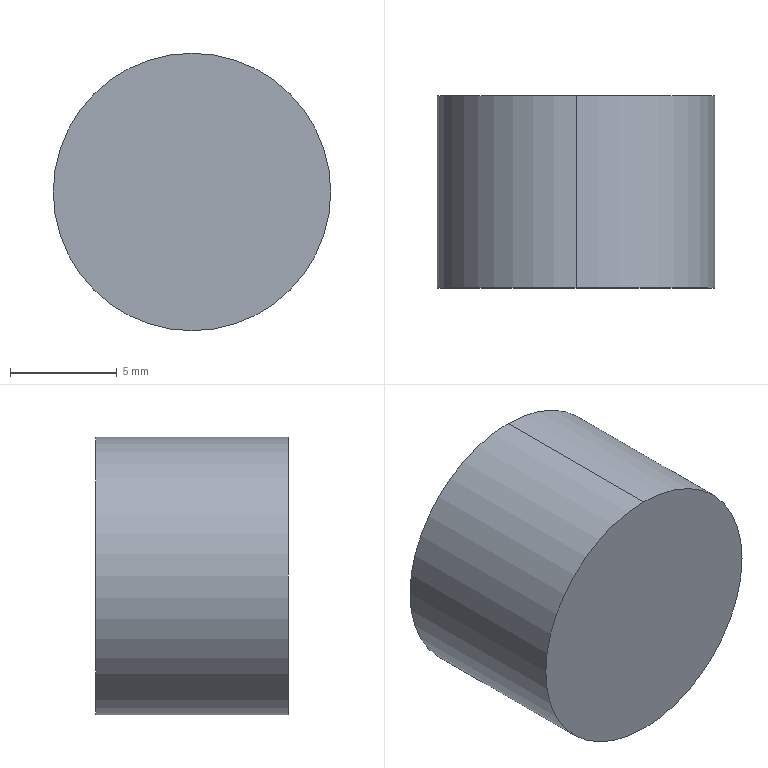Part | STEP file | 2-branch plug | 1 solid | 17 faces | box 13 x 9 x 13 mm | volume 992.021 mm3 | plane 15 | cylinder 2 | commonest cylinder face diameters 13 x2
STEP:
#1=CARTESIAN_POINT('',(0.,0.,0.));
#2=DIRECTION('',(0.,0.,1.));
#3=DIRECTION('',(1.,0.,0.));
#4=AXIS2_PLACEMENT_3D('',#1,#2,#3);
#5=CARTESIAN_POINT('',(0.,9.,6.5));
#6=VERTEX_POINT('',#5);
#7=CARTESIAN_POINT('',(0.,9.,-6.5));
#8=VERTEX_POINT('',#7);
#9=CARTESIAN_POINT('',(0.,9.,0.));
#10=DIRECTION('',(0.,1.,0.));
#11=DIRECTION('',(0.,0.,1.));
#12=AXIS2_PLACEMENT_3D('',#9,#10,#11);
#13=CIRCLE('',#12,6.5);
#14=CARTESIAN_POINT('',(0.,9.,0.));
#15=DIRECTION('',(0.,-1.,0.));
#16=DIRECTION('',(0.,0.,-1.));
#17=AXIS2_PLACEMENT_3D('',#14,#15,#16);
#18=CYLINDRICAL_SURFACE('',#17,6.5);
#19=CARTESIAN_POINT('',(3.142,0.));
#20=DIRECTION('',(-1.,0.));
#21=VECTOR('',#20,1.);
#22=LINE('',#19,#21);
#23=(GEOMETRIC_REPRESENTATION_CONTEXT(2)PARAMETRIC_REPRESENTATION_CONTEXT()REPRESENTATION_CONTEXT('',''));
#24=DEFINITIONAL_REPRESENTATION('',(#22),#23);
#25=PCURVE('',#18,#24);
#26=CARTESIAN_POINT('',(0.,9.,0.));
#27=DIRECTION('',(0.,1.,0.));
#28=DIRECTION('',(0.,0.,1.));
#29=AXIS2_PLACEMENT_3D('',#26,#27,#28);
#30=PLANE('',#29);
#31=CARTESIAN_POINT('',(0.,0.));
#32=DIRECTION('',(1.,0.));
#33=AXIS2_PLACEMENT_2D('',#31,#32);
#34=CIRCLE('',#33,6.5);
#35=(GEOMETRIC_REPRESENTATION_CONTEXT(2)PARAMETRIC_REPRESENTATION_CONTEXT()REPRESENTATION_CONTEXT('',''));
#36=DEFINITIONAL_REPRESENTATION('',(#34),#35);
#37=PCURVE('',#30,#36);
#38=SURFACE_CURVE('',#13,(#25,#37),.PCURVE_S1.);
#39=EDGE_CURVE('',#6,#8,#38,.T.);
#40=ORIENTED_EDGE('',*,*,#39,.F.);
#41=CARTESIAN_POINT('',(0.,0.,6.5));
#42=VERTEX_POINT('',#41);
#43=CARTESIAN_POINT('',(0.,9.,6.5));
#44=DIRECTION('',(0.,-1.,0.));
#45=VECTOR('',#44,1.);
#46=LINE('',#43,#45);
#47=CARTESIAN_POINT('',(3.142,0.));
#48=DIRECTION('',(0.,1.));
#49=VECTOR('',#48,1.);
#50=LINE('',#47,#49);
#51=(GEOMETRIC_REPRESENTATION_CONTEXT(2)PARAMETRIC_REPRESENTATION_CONTEXT()REPRESENTATION_CONTEXT('',''));
#52=DEFINITIONAL_REPRESENTATION('',(#50),#51);
#53=PCURVE('',#18,#52);
#54=CARTESIAN_POINT('',(0.,9.,0.));
#55=DIRECTION('',(0.,-1.,0.));
#56=DIRECTION('',(0.,0.,-1.));
#57=AXIS2_PLACEMENT_3D('',#54,#55,#56);
#58=CYLINDRICAL_SURFACE('',#57,6.5);
#59=CARTESIAN_POINT('',(3.142,0.));
#60=DIRECTION('',(0.,1.));
#61=VECTOR('',#60,1.);
#62=LINE('',#59,#61);
#63=(GEOMETRIC_REPRESENTATION_CONTEXT(2)PARAMETRIC_REPRESENTATION_CONTEXT()REPRESENTATION_CONTEXT('',''));
#64=DEFINITIONAL_REPRESENTATION('',(#62),#63);
#65=PCURVE('',#58,#64);
#66=SURFACE_CURVE('',#46,(#53,#65),.PCURVE_S1.);
#67=EDGE_CURVE('',#6,#42,#66,.T.);
#68=ORIENTED_EDGE('',*,*,#67,.T.);
#69=CARTESIAN_POINT('',(0.,0.,-6.5));
#70=VERTEX_POINT('',#69);
#71=CARTESIAN_POINT('',(0.,0.,0.));
#72=DIRECTION('',(0.,1.,0.));
#73=DIRECTION('',(0.,0.,1.));
#74=AXIS2_PLACEMENT_3D('',#71,#72,#73);
#75=CIRCLE('',#74,6.5);
#76=CARTESIAN_POINT('',(3.142,9.));
#77=DIRECTION('',(-1.,0.));
#78=VECTOR('',#77,1.);
#79=LINE('',#76,#78);
#80=(GEOMETRIC_REPRESENTATION_CONTEXT(2)PARAMETRIC_REPRESENTATION_CONTEXT()REPRESENTATION_CONTEXT('',''));
#81=DEFINITIONAL_REPRESENTATION('',(#79),#80);
#82=PCURVE('',#18,#81);
#83=CARTESIAN_POINT('',(0.,0.,0.));
#84=DIRECTION('',(0.,1.,0.));
#85=DIRECTION('',(0.,0.,1.));
#86=AXIS2_PLACEMENT_3D('',#83,#84,#85);
#87=PLANE('',#86);
#88=CARTESIAN_POINT('',(0.,0.));
#89=DIRECTION('',(1.,0.));
#90=AXIS2_PLACEMENT_2D('',#88,#89);
#91=CIRCLE('',#90,6.5);
#92=(GEOMETRIC_REPRESENTATION_CONTEXT(2)PARAMETRIC_REPRESENTATION_CONTEXT()REPRESENTATION_CONTEXT('',''));
#93=DEFINITIONAL_REPRESENTATION('',(#91),#92);
#94=PCURVE('',#87,#93);
#95=SURFACE_CURVE('',#75,(#82,#94),.PCURVE_S1.);
#96=EDGE_CURVE('',#42,#70,#95,.T.);
#97=ORIENTED_EDGE('',*,*,#96,.T.);
#98=CARTESIAN_POINT('',(0.,9.,-6.5));
#99=DIRECTION('',(0.,-1.,0.));
#100=VECTOR('',#99,1.);
#101=LINE('',#98,#100);
#102=CARTESIAN_POINT('',(0.,0.));
#103=DIRECTION('',(0.,1.));
#104=VECTOR('',#103,1.);
#105=LINE('',#102,#104);
#106=(GEOMETRIC_REPRESENTATION_CONTEXT(2)PARAMETRIC_REPRESENTATION_CONTEXT()REPRESENTATION_CONTEXT('',''));
#107=DEFINITIONAL_REPRESENTATION('',(#105),#106);
#108=PCURVE('',#18,#107);
#109=CARTESIAN_POINT('',(6.283,0.));
#110=DIRECTION('',(0.,1.));
#111=VECTOR('',#110,1.);
#112=LINE('',#109,#111);
#113=(GEOMETRIC_REPRESENTATION_CONTEXT(2)PARAMETRIC_REPRESENTATION_CONTEXT()REPRESENTATION_CONTEXT('',''));
#114=DEFINITIONAL_REPRESENTATION('',(#112),#113);
#115=PCURVE('',#58,#114);
#116=SURFACE_CURVE('',#101,(#108,#115),.PCURVE_S1.);
#117=EDGE_CURVE('',#8,#70,#116,.T.);
#118=ORIENTED_EDGE('',*,*,#117,.F.);
#119=EDGE_LOOP('',(#40,#68,#97,#118));
#120=FACE_BOUND('',#119,.T.);
#121=ADVANCED_FACE('',(#120),#18,.T.);
#122=ORIENTED_EDGE('',*,*,#67,.F.);
#123=CARTESIAN_POINT('',(0.,9.,0.));
#124=DIRECTION('',(0.,1.,0.));
#125=DIRECTION('',(0.,0.,1.));
#126=AXIS2_PLACEMENT_3D('',#123,#124,#125);
#127=CIRCLE('',#126,6.5);
#128=CARTESIAN_POINT('',(9.425,0.));
#129=DIRECTION('',(-1.,0.));
#130=VECTOR('',#129,1.);
#131=LINE('',#128,#130);
#132=(GEOMETRIC_REPRESENTATION_CONTEXT(2)PARAMETRIC_REPRESENTATION_CONTEXT()REPRESENTATION_CONTEXT('',''));
#133=DEFINITIONAL_REPRESENTATION('',(#131),#132);
#134=PCURVE('',#58,#133);
#135=CARTESIAN_POINT('',(0.,0.));
#136=DIRECTION('',(1.,0.));
#137=AXIS2_PLACEMENT_2D('',#135,#136);
#138=CIRCLE('',#137,6.5);
#139=(GEOMETRIC_REPRESENTATION_CONTEXT(2)PARAMETRIC_REPRESENTATION_CONTEXT()REPRESENTATION_CONTEXT('',''));
#140=DEFINITIONAL_REPRESENTATION('',(#138),#139);
#141=PCURVE('',#30,#140);
#142=SURFACE_CURVE('',#127,(#134,#141),.PCURVE_S1.);
#143=EDGE_CURVE('',#8,#6,#142,.T.);
#144=ORIENTED_EDGE('',*,*,#143,.F.);
#145=ORIENTED_EDGE('',*,*,#117,.T.);
#146=CARTESIAN_POINT('',(0.,0.,0.));
#147=DIRECTION('',(0.,1.,0.));
#148=DIRECTION('',(0.,0.,1.));
#149=AXIS2_PLACEMENT_3D('',#146,#147,#148);
#150=CIRCLE('',#149,6.5);
#151=CARTESIAN_POINT('',(9.425,9.));
#152=DIRECTION('',(-1.,0.));
#153=VECTOR('',#152,1.);
#154=LINE('',#151,#153);
#155=(GEOMETRIC_REPRESENTATION_CONTEXT(2)PARAMETRIC_REPRESENTATION_CONTEXT()REPRESENTATION_CONTEXT('',''));
#156=DEFINITIONAL_REPRESENTATION('',(#154),#155);
#157=PCURVE('',#58,#156);
#158=CARTESIAN_POINT('',(0.,0.));
#159=DIRECTION('',(1.,0.));
#160=AXIS2_PLACEMENT_2D('',#158,#159);
#161=CIRCLE('',#160,6.5);
#162=(GEOMETRIC_REPRESENTATION_CONTEXT(2)PARAMETRIC_REPRESENTATION_CONTEXT()REPRESENTATION_CONTEXT('',''));
#163=DEFINITIONAL_REPRESENTATION('',(#161),#162);
#164=PCURVE('',#87,#163);
#165=SURFACE_CURVE('',#150,(#157,#164),.PCURVE_S1.);
#166=EDGE_CURVE('',#70,#42,#165,.T.);
#167=ORIENTED_EDGE('',*,*,#166,.T.);
#168=EDGE_LOOP('',(#122,#144,#145,#167));
#169=FACE_BOUND('',#168,.T.);
#170=ADVANCED_FACE('',(#169),#58,.T.);
#171=CARTESIAN_POINT('',(-4.157,9.,0.04721));
#172=VERTEX_POINT('',#171);
#173=CARTESIAN_POINT('',(-2.119,9.,-3.576));
#174=VERTEX_POINT('',#173);
#175=CARTESIAN_POINT('',(-2.261,9.,-3.325));
#176=DIRECTION('',(0.4901,0.,-0.8716));
#177=VECTOR('',#176,1.);
#178=LINE('',#175,#177);
#179=CARTESIAN_POINT('',(-3.325,-2.261));
#180=DIRECTION('',(-0.8716,0.4901));
#181=VECTOR('',#180,1.);
#182=LINE('',#179,#181);
#183=(GEOMETRIC_REPRESENTATION_CONTEXT(2)PARAMETRIC_REPRESENTATION_CONTEXT()REPRESENTATION_CONTEXT('',''));
#184=DEFINITIONAL_REPRESENTATION('',(#182),#183);
#185=PCURVE('',#30,#184);
#186=CARTESIAN_POINT('',(-1.825,8.5,-3.079));
#187=DIRECTION('',(0.6163,0.7071,0.3466));
#188=DIRECTION('',(0.4901,0.,-0.8716));
#189=AXIS2_PLACEMENT_3D('',#186,#187,#188);
#190=PLANE('',#189);
#191=CARTESIAN_POINT('',(0.,0.7071));
#192=DIRECTION('',(1.,0.));
#193=VECTOR('',#192,1.);
#194=LINE('',#191,#193);
#195=(GEOMETRIC_REPRESENTATION_CONTEXT(2)PARAMETRIC_REPRESENTATION_CONTEXT()REPRESENTATION_CONTEXT('',''));
#196=DEFINITIONAL_REPRESENTATION('',(#194),#195);
#197=PCURVE('',#190,#196);
#198=SURFACE_CURVE('',#178,(#185,#197),.PCURVE_S1.);
#199=EDGE_CURVE('',#172,#174,#198,.T.);
#200=ORIENTED_EDGE('',*,*,#199,.T.);
#201=CARTESIAN_POINT('',(2.037,9.,-3.623));
#202=VERTEX_POINT('',#201);
#203=CARTESIAN_POINT('',(1.749,9.,-3.62));
#204=DIRECTION('',(0.9999,0.,-0.01136));
#205=VECTOR('',#204,1.);
#206=LINE('',#203,#205);
#207=CARTESIAN_POINT('',(-3.62,1.749));
#208=DIRECTION('',(-0.01136,0.9999));
#209=VECTOR('',#208,1.);
#210=LINE('',#207,#209);
#211=(GEOMETRIC_REPRESENTATION_CONTEXT(2)PARAMETRIC_REPRESENTATION_CONTEXT()REPRESENTATION_CONTEXT('',''));
#212=DEFINITIONAL_REPRESENTATION('',(#210),#211);
#213=PCURVE('',#30,#212);
#214=CARTESIAN_POINT('',(1.754,8.5,-3.12));
#215=DIRECTION('',(0.00803,0.7071,0.7071));
#216=DIRECTION('',(0.9999,0.,-0.01136));
#217=AXIS2_PLACEMENT_3D('',#214,#215,#216);
#218=PLANE('',#217);
#219=CARTESIAN_POINT('',(0.,0.7071));
#220=DIRECTION('',(1.,0.));
#221=VECTOR('',#220,1.);
#222=LINE('',#219,#221);
#223=(GEOMETRIC_REPRESENTATION_CONTEXT(2)PARAMETRIC_REPRESENTATION_CONTEXT()REPRESENTATION_CONTEXT('',''));
#224=DEFINITIONAL_REPRESENTATION('',(#222),#223);
#225=PCURVE('',#218,#224);
#226=SURFACE_CURVE('',#206,(#213,#225),.PCURVE_S1.);
#227=EDGE_CURVE('',#174,#202,#226,.T.);
#228=ORIENTED_EDGE('',*,*,#227,.T.);
#229=CARTESIAN_POINT('',(4.157,9.,-0.04721));
#230=VERTEX_POINT('',#229);
#231=CARTESIAN_POINT('',(4.009,9.,-0.2956));
#232=DIRECTION('',(0.5098,0.,0.8603));
#233=VECTOR('',#232,1.);
#234=LINE('',#231,#233);
#235=CARTESIAN_POINT('',(-0.2956,4.009));
#236=DIRECTION('',(0.8603,0.5098));
#237=VECTOR('',#236,1.);
#238=LINE('',#235,#237);
#239=(GEOMETRIC_REPRESENTATION_CONTEXT(2)PARAMETRIC_REPRESENTATION_CONTEXT()REPRESENTATION_CONTEXT('',''));
#240=DEFINITIONAL_REPRESENTATION('',(#238),#239);
#241=PCURVE('',#30,#240);
#242=CARTESIAN_POINT('',(3.579,8.5,-0.04065));
#243=DIRECTION('',(-0.6083,0.7071,0.3605));
#244=DIRECTION('',(0.5098,0.,0.8603));
#245=AXIS2_PLACEMENT_3D('',#242,#243,#244);
#246=PLANE('',#245);
#247=CARTESIAN_POINT('',(0.,0.7071));
#248=DIRECTION('',(1.,0.));
#249=VECTOR('',#248,1.);
#250=LINE('',#247,#249);
#251=(GEOMETRIC_REPRESENTATION_CONTEXT(2)PARAMETRIC_REPRESENTATION_CONTEXT()REPRESENTATION_CONTEXT('',''));
#252=DEFINITIONAL_REPRESENTATION('',(#250),#251);
#253=PCURVE('',#246,#252);
#254=SURFACE_CURVE('',#234,(#241,#253),.PCURVE_S1.);
#255=EDGE_CURVE('',#202,#230,#254,.T.);
#256=ORIENTED_EDGE('',*,*,#255,.T.);
#257=CARTESIAN_POINT('',(2.119,9.,3.576));
#258=VERTEX_POINT('',#257);
#259=CARTESIAN_POINT('',(2.261,9.,3.325));
#260=DIRECTION('',(-0.4901,0.,0.8716));
#261=VECTOR('',#260,1.);
#262=LINE('',#259,#261);
#263=CARTESIAN_POINT('',(3.325,2.261));
#264=DIRECTION('',(0.8716,-0.4901));
#265=VECTOR('',#264,1.);
#266=LINE('',#263,#265);
#267=(GEOMETRIC_REPRESENTATION_CONTEXT(2)PARAMETRIC_REPRESENTATION_CONTEXT()REPRESENTATION_CONTEXT('',''));
#268=DEFINITIONAL_REPRESENTATION('',(#266),#267);
#269=PCURVE('',#30,#268);
#270=CARTESIAN_POINT('',(1.825,8.5,3.079));
#271=DIRECTION('',(-0.6163,0.7071,-0.3466));
#272=DIRECTION('',(-0.4901,0.,0.8716));
#273=AXIS2_PLACEMENT_3D('',#270,#271,#272);
#274=PLANE('',#273);
#275=CARTESIAN_POINT('',(0.,0.7071));
#276=DIRECTION('',(1.,0.));
#277=VECTOR('',#276,1.);
#278=LINE('',#275,#277);
#279=(GEOMETRIC_REPRESENTATION_CONTEXT(2)PARAMETRIC_REPRESENTATION_CONTEXT()REPRESENTATION_CONTEXT('',''));
#280=DEFINITIONAL_REPRESENTATION('',(#278),#279);
#281=PCURVE('',#274,#280);
#282=SURFACE_CURVE('',#262,(#269,#281),.PCURVE_S1.);
#283=EDGE_CURVE('',#230,#258,#282,.T.);
#284=ORIENTED_EDGE('',*,*,#283,.T.);
#285=CARTESIAN_POINT('',(-2.037,9.,3.623));
#286=VERTEX_POINT('',#285);
#287=CARTESIAN_POINT('',(-1.749,9.,3.62));
#288=DIRECTION('',(-0.9999,0.,0.01136));
#289=VECTOR('',#288,1.);
#290=LINE('',#287,#289);
#291=CARTESIAN_POINT('',(3.62,-1.749));
#292=DIRECTION('',(0.01136,-0.9999));
#293=VECTOR('',#292,1.);
#294=LINE('',#291,#293);
#295=(GEOMETRIC_REPRESENTATION_CONTEXT(2)PARAMETRIC_REPRESENTATION_CONTEXT()REPRESENTATION_CONTEXT('',''));
#296=DEFINITIONAL_REPRESENTATION('',(#294),#295);
#297=PCURVE('',#30,#296);
#298=CARTESIAN_POINT('',(-1.754,8.5,3.12));
#299=DIRECTION('',(-0.00803,0.7071,-0.7071));
#300=DIRECTION('',(-0.9999,0.,0.01136));
#301=AXIS2_PLACEMENT_3D('',#298,#299,#300);
#302=PLANE('',#301);
#303=CARTESIAN_POINT('',(0.,0.7071));
#304=DIRECTION('',(1.,0.));
#305=VECTOR('',#304,1.);
#306=LINE('',#303,#305);
#307=(GEOMETRIC_REPRESENTATION_CONTEXT(2)PARAMETRIC_REPRESENTATION_CONTEXT()REPRESENTATION_CONTEXT('',''));
#308=DEFINITIONAL_REPRESENTATION('',(#306),#307);
#309=PCURVE('',#302,#308);
#310=SURFACE_CURVE('',#290,(#297,#309),.PCURVE_S1.);
#311=EDGE_CURVE('',#258,#286,#310,.T.);
#312=ORIENTED_EDGE('',*,*,#311,.T.);
#313=CARTESIAN_POINT('',(-4.009,9.,0.2956));
#314=DIRECTION('',(-0.5098,0.,-0.8603));
#315=VECTOR('',#314,1.);
#316=LINE('',#313,#315);
#317=CARTESIAN_POINT('',(0.2956,-4.009));
#318=DIRECTION('',(-0.8603,-0.5098));
#319=VECTOR('',#318,1.);
#320=LINE('',#317,#319);
#321=(GEOMETRIC_REPRESENTATION_CONTEXT(2)PARAMETRIC_REPRESENTATION_CONTEXT()REPRESENTATION_CONTEXT('',''));
#322=DEFINITIONAL_REPRESENTATION('',(#320),#321);
#323=PCURVE('',#30,#322);
#324=CARTESIAN_POINT('',(-3.579,8.5,0.04065));
#325=DIRECTION('',(0.6083,0.7071,-0.3605));
#326=DIRECTION('',(-0.5098,0.,-0.8603));
#327=AXIS2_PLACEMENT_3D('',#324,#325,#326);
#328=PLANE('',#327);
#329=CARTESIAN_POINT('',(0.,0.7071));
#330=DIRECTION('',(1.,0.));
#331=VECTOR('',#330,1.);
#332=LINE('',#329,#331);
#333=(GEOMETRIC_REPRESENTATION_CONTEXT(2)PARAMETRIC_REPRESENTATION_CONTEXT()REPRESENTATION_CONTEXT('',''));
#334=DEFINITIONAL_REPRESENTATION('',(#332),#333);
#335=PCURVE('',#328,#334);
#336=SURFACE_CURVE('',#316,(#323,#335),.PCURVE_S1.);
#337=EDGE_CURVE('',#286,#172,#336,.T.);
#338=ORIENTED_EDGE('',*,*,#337,.T.);
#339=EDGE_LOOP('',(#200,#228,#256,#284,#312,#338));
#340=FACE_BOUND('',#339,.T.);
#341=ORIENTED_EDGE('',*,*,#143,.T.);
#342=ORIENTED_EDGE('',*,*,#39,.T.);
#343=EDGE_LOOP('',(#341,#342));
#344=FACE_BOUND('',#343,.T.);
#345=ADVANCED_FACE('',(#340,#344),#30,.T.);
#346=ORIENTED_EDGE('',*,*,#166,.F.);
#347=ORIENTED_EDGE('',*,*,#96,.F.);
#348=EDGE_LOOP('',(#346,#347));
#349=FACE_BOUND('',#348,.T.);
#350=ADVANCED_FACE('',(#349),#87,.F.);
#351=CARTESIAN_POINT('',(-1.754,3.,3.12));
#352=VERTEX_POINT('',#351);
#353=CARTESIAN_POINT('',(-1.754,8.5,3.12));
#354=VERTEX_POINT('',#353);
#355=CARTESIAN_POINT('',(-1.754,3.,3.12));
#356=DIRECTION('',(0.,1.,0.));
#357=VECTOR('',#356,1.);
#358=LINE('',#355,#357);
#359=CARTESIAN_POINT('',(-1.754,3.,3.12));
#360=DIRECTION('',(0.01136,0.,0.9999));
#361=DIRECTION('',(0.9999,0.,-0.01136));
#362=AXIS2_PLACEMENT_3D('',#359,#360,#361);
#363=PLANE('',#362);
#364=CARTESIAN_POINT('',(0.,0.));
#365=DIRECTION('',(0.,1.));
#366=VECTOR('',#365,1.);
#367=LINE('',#364,#366);
#368=(GEOMETRIC_REPRESENTATION_CONTEXT(2)PARAMETRIC_REPRESENTATION_CONTEXT()REPRESENTATION_CONTEXT('',''));
#369=DEFINITIONAL_REPRESENTATION('',(#367),#368);
#370=PCURVE('',#363,#369);
#371=CARTESIAN_POINT('',(-3.579,3.,0.04065));
#372=DIRECTION('',(-0.8603,0.,0.5098));
#373=DIRECTION('',(0.5098,0.,0.8603));
#374=AXIS2_PLACEMENT_3D('',#371,#372,#373);
#375=PLANE('',#374);
#376=CARTESIAN_POINT('',(3.58,0.));
#377=DIRECTION('',(0.,1.));
#378=VECTOR('',#377,1.);
#379=LINE('',#376,#378);
#380=(GEOMETRIC_REPRESENTATION_CONTEXT(2)PARAMETRIC_REPRESENTATION_CONTEXT()REPRESENTATION_CONTEXT('',''));
#381=DEFINITIONAL_REPRESENTATION('',(#379),#380);
#382=PCURVE('',#375,#381);
#383=SURFACE_CURVE('',#358,(#370,#382),.PCURVE_S1.);
#384=EDGE_CURVE('',#352,#354,#383,.T.);
#385=ORIENTED_EDGE('',*,*,#384,.T.);
#386=CARTESIAN_POINT('',(1.825,8.5,3.079));
#387=VERTEX_POINT('',#386);
#388=CARTESIAN_POINT('',(1.825,8.5,3.079));
#389=DIRECTION('',(0.9999,0.,-0.01136));
#390=VECTOR('',#389,1.);
#391=LINE('',#388,#390);
#392=CARTESIAN_POINT('',(3.58,5.5));
#393=DIRECTION('',(1.,0.));
#394=VECTOR('',#393,1.);
#395=LINE('',#392,#394);
#396=(GEOMETRIC_REPRESENTATION_CONTEXT(2)PARAMETRIC_REPRESENTATION_CONTEXT()REPRESENTATION_CONTEXT('',''));
#397=DEFINITIONAL_REPRESENTATION('',(#395),#396);
#398=PCURVE('',#363,#397);
#399=CARTESIAN_POINT('',(-3.58,0.));
#400=DIRECTION('',(-1.,0.));
#401=VECTOR('',#400,1.);
#402=LINE('',#399,#401);
#403=(GEOMETRIC_REPRESENTATION_CONTEXT(2)PARAMETRIC_REPRESENTATION_CONTEXT()REPRESENTATION_CONTEXT('',''));
#404=DEFINITIONAL_REPRESENTATION('',(#402),#403);
#405=PCURVE('',#302,#404);
#406=SURFACE_CURVE('',#391,(#398,#405),.PCURVE_S1.);
#407=EDGE_CURVE('',#354,#387,#406,.T.);
#408=ORIENTED_EDGE('',*,*,#407,.T.);
#409=CARTESIAN_POINT('',(1.825,3.,3.079));
#410=VERTEX_POINT('',#409);
#411=CARTESIAN_POINT('',(1.825,3.,3.079));
#412=DIRECTION('',(0.,1.,0.));
#413=VECTOR('',#412,1.);
#414=LINE('',#411,#413);
#415=CARTESIAN_POINT('',(3.58,0.));
#416=DIRECTION('',(0.,1.));
#417=VECTOR('',#416,1.);
#418=LINE('',#415,#417);
#419=(GEOMETRIC_REPRESENTATION_CONTEXT(2)PARAMETRIC_REPRESENTATION_CONTEXT()REPRESENTATION_CONTEXT('',''));
#420=DEFINITIONAL_REPRESENTATION('',(#418),#419);
#421=PCURVE('',#363,#420);
#422=CARTESIAN_POINT('',(1.825,3.,3.079));
#423=DIRECTION('',(0.8716,0.,0.4901));
#424=DIRECTION('',(0.4901,0.,-0.8716));
#425=AXIS2_PLACEMENT_3D('',#422,#423,#424);
#426=PLANE('',#425);
#427=CARTESIAN_POINT('',(0.,0.));
#428=DIRECTION('',(0.,1.));
#429=VECTOR('',#428,1.);
#430=LINE('',#427,#429);
#431=(GEOMETRIC_REPRESENTATION_CONTEXT(2)PARAMETRIC_REPRESENTATION_CONTEXT()REPRESENTATION_CONTEXT('',''));
#432=DEFINITIONAL_REPRESENTATION('',(#430),#431);
#433=PCURVE('',#426,#432);
#434=SURFACE_CURVE('',#414,(#421,#433),.PCURVE_S1.);
#435=EDGE_CURVE('',#410,#387,#434,.T.);
#436=ORIENTED_EDGE('',*,*,#435,.F.);
#437=CARTESIAN_POINT('',(-1.754,3.,3.12));
#438=DIRECTION('',(0.9999,0.,-0.01136));
#439=VECTOR('',#438,1.);
#440=LINE('',#437,#439);
#441=CARTESIAN_POINT('',(0.,0.));
#442=DIRECTION('',(1.,0.));
#443=VECTOR('',#442,1.);
#444=LINE('',#441,#443);
#445=(GEOMETRIC_REPRESENTATION_CONTEXT(2)PARAMETRIC_REPRESENTATION_CONTEXT()REPRESENTATION_CONTEXT('',''));
#446=DEFINITIONAL_REPRESENTATION('',(#444),#445);
#447=PCURVE('',#363,#446);
#448=CARTESIAN_POINT('',(0.,3.,0.));
#449=DIRECTION('',(0.,1.,0.));
#450=DIRECTION('',(0.,0.,1.));
#451=AXIS2_PLACEMENT_3D('',#448,#449,#450);
#452=PLANE('',#451);
#453=CARTESIAN_POINT('',(3.12,-1.754));
#454=DIRECTION('',(-0.01136,0.9999));
#455=VECTOR('',#454,1.);
#456=LINE('',#453,#455);
#457=(GEOMETRIC_REPRESENTATION_CONTEXT(2)PARAMETRIC_REPRESENTATION_CONTEXT()REPRESENTATION_CONTEXT('',''));
#458=DEFINITIONAL_REPRESENTATION('',(#456),#457);
#459=PCURVE('',#452,#458);
#460=SURFACE_CURVE('',#440,(#447,#459),.PCURVE_S1.);
#461=EDGE_CURVE('',#352,#410,#460,.T.);
#462=ORIENTED_EDGE('',*,*,#461,.F.);
#463=EDGE_LOOP('',(#385,#408,#436,#462));
#464=FACE_BOUND('',#463,.T.);
#465=ADVANCED_FACE('',(#464),#363,.F.);
#466=CARTESIAN_POINT('',(-3.579,3.,0.04065));
#467=VERTEX_POINT('',#466);
#468=CARTESIAN_POINT('',(-3.579,8.5,0.04065));
#469=VERTEX_POINT('',#468);
#470=CARTESIAN_POINT('',(-3.579,3.,0.04065));
#471=DIRECTION('',(0.,1.,0.));
#472=VECTOR('',#471,1.);
#473=LINE('',#470,#472);
#474=CARTESIAN_POINT('',(0.,0.));
#475=DIRECTION('',(0.,1.));
#476=VECTOR('',#475,1.);
#477=LINE('',#474,#476);
#478=(GEOMETRIC_REPRESENTATION_CONTEXT(2)PARAMETRIC_REPRESENTATION_CONTEXT()REPRESENTATION_CONTEXT('',''));
#479=DEFINITIONAL_REPRESENTATION('',(#477),#478);
#480=PCURVE('',#375,#479);
#481=CARTESIAN_POINT('',(-1.825,3.,-3.079));
#482=DIRECTION('',(-0.8716,0.,-0.4901));
#483=DIRECTION('',(-0.4901,0.,0.8716));
#484=AXIS2_PLACEMENT_3D('',#481,#482,#483);
#485=PLANE('',#484);
#486=CARTESIAN_POINT('',(3.58,0.));
#487=DIRECTION('',(0.,1.));
#488=VECTOR('',#487,1.);
#489=LINE('',#486,#488);
#490=(GEOMETRIC_REPRESENTATION_CONTEXT(2)PARAMETRIC_REPRESENTATION_CONTEXT()REPRESENTATION_CONTEXT('',''));
#491=DEFINITIONAL_REPRESENTATION('',(#489),#490);
#492=PCURVE('',#485,#491);
#493=SURFACE_CURVE('',#473,(#480,#492),.PCURVE_S1.);
#494=EDGE_CURVE('',#467,#469,#493,.T.);
#495=ORIENTED_EDGE('',*,*,#494,.T.);
#496=CARTESIAN_POINT('',(-1.754,8.5,3.12));
#497=DIRECTION('',(0.5098,0.,0.8603));
#498=VECTOR('',#497,1.);
#499=LINE('',#496,#498);
#500=CARTESIAN_POINT('',(3.58,5.5));
#501=DIRECTION('',(1.,0.));
#502=VECTOR('',#501,1.);
#503=LINE('',#500,#502);
#504=(GEOMETRIC_REPRESENTATION_CONTEXT(2)PARAMETRIC_REPRESENTATION_CONTEXT()REPRESENTATION_CONTEXT('',''));
#505=DEFINITIONAL_REPRESENTATION('',(#503),#504);
#506=PCURVE('',#375,#505);
#507=CARTESIAN_POINT('',(-3.58,0.));
#508=DIRECTION('',(-1.,0.));
#509=VECTOR('',#508,1.);
#510=LINE('',#507,#509);
#511=(GEOMETRIC_REPRESENTATION_CONTEXT(2)PARAMETRIC_REPRESENTATION_CONTEXT()REPRESENTATION_CONTEXT('',''));
#512=DEFINITIONAL_REPRESENTATION('',(#510),#511);
#513=PCURVE('',#328,#512);
#514=SURFACE_CURVE('',#499,(#506,#513),.PCURVE_S1.);
#515=EDGE_CURVE('',#469,#354,#514,.T.);
#516=ORIENTED_EDGE('',*,*,#515,.T.);
#517=ORIENTED_EDGE('',*,*,#384,.F.);
#518=CARTESIAN_POINT('',(-3.579,3.,0.04065));
#519=DIRECTION('',(0.5098,0.,0.8603));
#520=VECTOR('',#519,1.);
#521=LINE('',#518,#520);
#522=CARTESIAN_POINT('',(0.,0.));
#523=DIRECTION('',(1.,0.));
#524=VECTOR('',#523,1.);
#525=LINE('',#522,#524);
#526=(GEOMETRIC_REPRESENTATION_CONTEXT(2)PARAMETRIC_REPRESENTATION_CONTEXT()REPRESENTATION_CONTEXT('',''));
#527=DEFINITIONAL_REPRESENTATION('',(#525),#526);
#528=PCURVE('',#375,#527);
#529=CARTESIAN_POINT('',(0.04065,-3.579));
#530=DIRECTION('',(0.8603,0.5098));
#531=VECTOR('',#530,1.);
#532=LINE('',#529,#531);
#533=(GEOMETRIC_REPRESENTATION_CONTEXT(2)PARAMETRIC_REPRESENTATION_CONTEXT()REPRESENTATION_CONTEXT('',''));
#534=DEFINITIONAL_REPRESENTATION('',(#532),#533);
#535=PCURVE('',#452,#534);
#536=SURFACE_CURVE('',#521,(#528,#535),.PCURVE_S1.);
#537=EDGE_CURVE('',#467,#352,#536,.T.);
#538=ORIENTED_EDGE('',*,*,#537,.F.);
#539=EDGE_LOOP('',(#495,#516,#517,#538));
#540=FACE_BOUND('',#539,.T.);
#541=ADVANCED_FACE('',(#540),#375,.F.);
#542=CARTESIAN_POINT('',(-1.825,3.,-3.079));
#543=VERTEX_POINT('',#542);
#544=CARTESIAN_POINT('',(-1.825,8.5,-3.079));
#545=VERTEX_POINT('',#544);
#546=CARTESIAN_POINT('',(-1.825,3.,-3.079));
#547=DIRECTION('',(0.,1.,0.));
#548=VECTOR('',#547,1.);
#549=LINE('',#546,#548);
#550=CARTESIAN_POINT('',(0.,0.));
#551=DIRECTION('',(0.,1.));
#552=VECTOR('',#551,1.);
#553=LINE('',#550,#552);
#554=(GEOMETRIC_REPRESENTATION_CONTEXT(2)PARAMETRIC_REPRESENTATION_CONTEXT()REPRESENTATION_CONTEXT('',''));
#555=DEFINITIONAL_REPRESENTATION('',(#553),#554);
#556=PCURVE('',#485,#555);
#557=CARTESIAN_POINT('',(1.754,3.,-3.12));
#558=DIRECTION('',(-0.01136,0.,-0.9999));
#559=DIRECTION('',(-0.9999,0.,0.01136));
#560=AXIS2_PLACEMENT_3D('',#557,#558,#559);
#561=PLANE('',#560);
#562=CARTESIAN_POINT('',(3.58,0.));
#563=DIRECTION('',(0.,1.));
#564=VECTOR('',#563,1.);
#565=LINE('',#562,#564);
#566=(GEOMETRIC_REPRESENTATION_CONTEXT(2)PARAMETRIC_REPRESENTATION_CONTEXT()REPRESENTATION_CONTEXT('',''));
#567=DEFINITIONAL_REPRESENTATION('',(#565),#566);
#568=PCURVE('',#561,#567);
#569=SURFACE_CURVE('',#549,(#556,#568),.PCURVE_S1.);
#570=EDGE_CURVE('',#543,#545,#569,.T.);
#571=ORIENTED_EDGE('',*,*,#570,.T.);
#572=CARTESIAN_POINT('',(-3.579,8.5,0.04065));
#573=DIRECTION('',(-0.4901,0.,0.8716));
#574=VECTOR('',#573,1.);
#575=LINE('',#572,#574);
#576=CARTESIAN_POINT('',(3.58,5.5));
#577=DIRECTION('',(1.,0.));
#578=VECTOR('',#577,1.);
#579=LINE('',#576,#578);
#580=(GEOMETRIC_REPRESENTATION_CONTEXT(2)PARAMETRIC_REPRESENTATION_CONTEXT()REPRESENTATION_CONTEXT('',''));
#581=DEFINITIONAL_REPRESENTATION('',(#579),#580);
#582=PCURVE('',#485,#581);
#583=CARTESIAN_POINT('',(-3.58,0.));
#584=DIRECTION('',(-1.,0.));
#585=VECTOR('',#584,1.);
#586=LINE('',#583,#585);
#587=(GEOMETRIC_REPRESENTATION_CONTEXT(2)PARAMETRIC_REPRESENTATION_CONTEXT()REPRESENTATION_CONTEXT('',''));
#588=DEFINITIONAL_REPRESENTATION('',(#586),#587);
#589=PCURVE('',#190,#588);
#590=SURFACE_CURVE('',#575,(#582,#589),.PCURVE_S1.);
#591=EDGE_CURVE('',#545,#469,#590,.T.);
#592=ORIENTED_EDGE('',*,*,#591,.T.);
#593=ORIENTED_EDGE('',*,*,#494,.F.);
#594=CARTESIAN_POINT('',(-1.825,3.,-3.079));
#595=DIRECTION('',(-0.4901,0.,0.8716));
#596=VECTOR('',#595,1.);
#597=LINE('',#594,#596);
#598=CARTESIAN_POINT('',(0.,0.));
#599=DIRECTION('',(1.,0.));
#600=VECTOR('',#599,1.);
#601=LINE('',#598,#600);
#602=(GEOMETRIC_REPRESENTATION_CONTEXT(2)PARAMETRIC_REPRESENTATION_CONTEXT()REPRESENTATION_CONTEXT('',''));
#603=DEFINITIONAL_REPRESENTATION('',(#601),#602);
#604=PCURVE('',#485,#603);
#605=CARTESIAN_POINT('',(-3.079,-1.825));
#606=DIRECTION('',(0.8716,-0.4901));
#607=VECTOR('',#606,1.);
#608=LINE('',#605,#607);
#609=(GEOMETRIC_REPRESENTATION_CONTEXT(2)PARAMETRIC_REPRESENTATION_CONTEXT()REPRESENTATION_CONTEXT('',''));
#610=DEFINITIONAL_REPRESENTATION('',(#608),#609);
#611=PCURVE('',#452,#610);
#612=SURFACE_CURVE('',#597,(#604,#611),.PCURVE_S1.);
#613=EDGE_CURVE('',#543,#467,#612,.T.);
#614=ORIENTED_EDGE('',*,*,#613,.F.);
#615=EDGE_LOOP('',(#571,#592,#593,#614));
#616=FACE_BOUND('',#615,.T.);
#617=ADVANCED_FACE('',(#616),#485,.F.);
#618=CARTESIAN_POINT('',(1.754,3.,-3.12));
#619=VERTEX_POINT('',#618);
#620=CARTESIAN_POINT('',(1.754,8.5,-3.12));
#621=VERTEX_POINT('',#620);
#622=CARTESIAN_POINT('',(1.754,3.,-3.12));
#623=DIRECTION('',(0.,1.,0.));
#624=VECTOR('',#623,1.);
#625=LINE('',#622,#624);
#626=CARTESIAN_POINT('',(0.,0.));
#627=DIRECTION('',(0.,1.));
#628=VECTOR('',#627,1.);
#629=LINE('',#626,#628);
#630=(GEOMETRIC_REPRESENTATION_CONTEXT(2)PARAMETRIC_REPRESENTATION_CONTEXT()REPRESENTATION_CONTEXT('',''));
#631=DEFINITIONAL_REPRESENTATION('',(#629),#630);
#632=PCURVE('',#561,#631);
#633=CARTESIAN_POINT('',(3.579,3.,-0.04065));
#634=DIRECTION('',(0.8603,0.,-0.5098));
#635=DIRECTION('',(-0.5098,0.,-0.8603));
#636=AXIS2_PLACEMENT_3D('',#633,#634,#635);
#637=PLANE('',#636);
#638=CARTESIAN_POINT('',(3.58,0.));
#639=DIRECTION('',(0.,1.));
#640=VECTOR('',#639,1.);
#641=LINE('',#638,#640);
#642=(GEOMETRIC_REPRESENTATION_CONTEXT(2)PARAMETRIC_REPRESENTATION_CONTEXT()REPRESENTATION_CONTEXT('',''));
#643=DEFINITIONAL_REPRESENTATION('',(#641),#642);
#644=PCURVE('',#637,#643);
#645=SURFACE_CURVE('',#625,(#632,#644),.PCURVE_S1.);
#646=EDGE_CURVE('',#619,#621,#645,.T.);
#647=ORIENTED_EDGE('',*,*,#646,.T.);
#648=CARTESIAN_POINT('',(-1.825,8.5,-3.079));
#649=DIRECTION('',(-0.9999,0.,0.01136));
#650=VECTOR('',#649,1.);
#651=LINE('',#648,#650);
#652=CARTESIAN_POINT('',(3.58,5.5));
#653=DIRECTION('',(1.,0.));
#654=VECTOR('',#653,1.);
#655=LINE('',#652,#654);
#656=(GEOMETRIC_REPRESENTATION_CONTEXT(2)PARAMETRIC_REPRESENTATION_CONTEXT()REPRESENTATION_CONTEXT('',''));
#657=DEFINITIONAL_REPRESENTATION('',(#655),#656);
#658=PCURVE('',#561,#657);
#659=CARTESIAN_POINT('',(-3.58,0.));
#660=DIRECTION('',(-1.,0.));
#661=VECTOR('',#660,1.);
#662=LINE('',#659,#661);
#663=(GEOMETRIC_REPRESENTATION_CONTEXT(2)PARAMETRIC_REPRESENTATION_CONTEXT()REPRESENTATION_CONTEXT('',''));
#664=DEFINITIONAL_REPRESENTATION('',(#662),#663);
#665=PCURVE('',#218,#664);
#666=SURFACE_CURVE('',#651,(#658,#665),.PCURVE_S1.);
#667=EDGE_CURVE('',#621,#545,#666,.T.);
#668=ORIENTED_EDGE('',*,*,#667,.T.);
#669=ORIENTED_EDGE('',*,*,#570,.F.);
#670=CARTESIAN_POINT('',(1.754,3.,-3.12));
#671=DIRECTION('',(-0.9999,0.,0.01136));
#672=VECTOR('',#671,1.);
#673=LINE('',#670,#672);
#674=CARTESIAN_POINT('',(0.,0.));
#675=DIRECTION('',(1.,0.));
#676=VECTOR('',#675,1.);
#677=LINE('',#674,#676);
#678=(GEOMETRIC_REPRESENTATION_CONTEXT(2)PARAMETRIC_REPRESENTATION_CONTEXT()REPRESENTATION_CONTEXT('',''));
#679=DEFINITIONAL_REPRESENTATION('',(#677),#678);
#680=PCURVE('',#561,#679);
#681=CARTESIAN_POINT('',(-3.12,1.754));
#682=DIRECTION('',(0.01136,-0.9999));
#683=VECTOR('',#682,1.);
#684=LINE('',#681,#683);
#685=(GEOMETRIC_REPRESENTATION_CONTEXT(2)PARAMETRIC_REPRESENTATION_CONTEXT()REPRESENTATION_CONTEXT('',''));
#686=DEFINITIONAL_REPRESENTATION('',(#684),#685);
#687=PCURVE('',#452,#686);
#688=SURFACE_CURVE('',#673,(#680,#687),.PCURVE_S1.);
#689=EDGE_CURVE('',#619,#543,#688,.T.);
#690=ORIENTED_EDGE('',*,*,#689,.F.);
#691=EDGE_LOOP('',(#647,#668,#669,#690));
#692=FACE_BOUND('',#691,.T.);
#693=ADVANCED_FACE('',(#692),#561,.F.);
#694=CARTESIAN_POINT('',(3.579,3.,-0.04065));
#695=VERTEX_POINT('',#694);
#696=CARTESIAN_POINT('',(3.579,8.5,-0.04065));
#697=VERTEX_POINT('',#696);
#698=CARTESIAN_POINT('',(3.579,3.,-0.04065));
#699=DIRECTION('',(0.,1.,0.));
#700=VECTOR('',#699,1.);
#701=LINE('',#698,#700);
#702=CARTESIAN_POINT('',(0.,0.));
#703=DIRECTION('',(0.,1.));
#704=VECTOR('',#703,1.);
#705=LINE('',#702,#704);
#706=(GEOMETRIC_REPRESENTATION_CONTEXT(2)PARAMETRIC_REPRESENTATION_CONTEXT()REPRESENTATION_CONTEXT('',''));
#707=DEFINITIONAL_REPRESENTATION('',(#705),#706);
#708=PCURVE('',#637,#707);
#709=CARTESIAN_POINT('',(3.58,0.));
#710=DIRECTION('',(0.,1.));
#711=VECTOR('',#710,1.);
#712=LINE('',#709,#711);
#713=(GEOMETRIC_REPRESENTATION_CONTEXT(2)PARAMETRIC_REPRESENTATION_CONTEXT()REPRESENTATION_CONTEXT('',''));
#714=DEFINITIONAL_REPRESENTATION('',(#712),#713);
#715=PCURVE('',#426,#714);
#716=SURFACE_CURVE('',#701,(#708,#715),.PCURVE_S1.);
#717=EDGE_CURVE('',#695,#697,#716,.T.);
#718=ORIENTED_EDGE('',*,*,#717,.T.);
#719=CARTESIAN_POINT('',(1.754,8.5,-3.12));
#720=DIRECTION('',(-0.5098,0.,-0.8603));
#721=VECTOR('',#720,1.);
#722=LINE('',#719,#721);
#723=CARTESIAN_POINT('',(3.58,5.5));
#724=DIRECTION('',(1.,0.));
#725=VECTOR('',#724,1.);
#726=LINE('',#723,#725);
#727=(GEOMETRIC_REPRESENTATION_CONTEXT(2)PARAMETRIC_REPRESENTATION_CONTEXT()REPRESENTATION_CONTEXT('',''));
#728=DEFINITIONAL_REPRESENTATION('',(#726),#727);
#729=PCURVE('',#637,#728);
#730=CARTESIAN_POINT('',(-3.58,0.));
#731=DIRECTION('',(-1.,0.));
#732=VECTOR('',#731,1.);
#733=LINE('',#730,#732);
#734=(GEOMETRIC_REPRESENTATION_CONTEXT(2)PARAMETRIC_REPRESENTATION_CONTEXT()REPRESENTATION_CONTEXT('',''));
#735=DEFINITIONAL_REPRESENTATION('',(#733),#734);
#736=PCURVE('',#246,#735);
#737=SURFACE_CURVE('',#722,(#729,#736),.PCURVE_S1.);
#738=EDGE_CURVE('',#697,#621,#737,.T.);
#739=ORIENTED_EDGE('',*,*,#738,.T.);
#740=ORIENTED_EDGE('',*,*,#646,.F.);
#741=CARTESIAN_POINT('',(3.579,3.,-0.04065));
#742=DIRECTION('',(-0.5098,0.,-0.8603));
#743=VECTOR('',#742,1.);
#744=LINE('',#741,#743);
#745=CARTESIAN_POINT('',(0.,0.));
#746=DIRECTION('',(1.,0.));
#747=VECTOR('',#746,1.);
#748=LINE('',#745,#747);
#749=(GEOMETRIC_REPRESENTATION_CONTEXT(2)PARAMETRIC_REPRESENTATION_CONTEXT()REPRESENTATION_CONTEXT('',''));
#750=DEFINITIONAL_REPRESENTATION('',(#748),#749);
#751=PCURVE('',#637,#750);
#752=CARTESIAN_POINT('',(-0.04065,3.579));
#753=DIRECTION('',(-0.8603,-0.5098));
#754=VECTOR('',#753,1.);
#755=LINE('',#752,#754);
#756=(GEOMETRIC_REPRESENTATION_CONTEXT(2)PARAMETRIC_REPRESENTATION_CONTEXT()REPRESENTATION_CONTEXT('',''));
#757=DEFINITIONAL_REPRESENTATION('',(#755),#756);
#758=PCURVE('',#452,#757);
#759=SURFACE_CURVE('',#744,(#751,#758),.PCURVE_S1.);
#760=EDGE_CURVE('',#695,#619,#759,.T.);
#761=ORIENTED_EDGE('',*,*,#760,.F.);
#762=EDGE_LOOP('',(#718,#739,#740,#761));
#763=FACE_BOUND('',#762,.T.);
#764=ADVANCED_FACE('',(#763),#637,.F.);
#765=ORIENTED_EDGE('',*,*,#435,.T.);
#766=CARTESIAN_POINT('',(3.579,8.5,-0.04065));
#767=DIRECTION('',(0.4901,0.,-0.8716));
#768=VECTOR('',#767,1.);
#769=LINE('',#766,#768);
#770=CARTESIAN_POINT('',(3.58,5.5));
#771=DIRECTION('',(1.,0.));
#772=VECTOR('',#771,1.);
#773=LINE('',#770,#772);
#774=(GEOMETRIC_REPRESENTATION_CONTEXT(2)PARAMETRIC_REPRESENTATION_CONTEXT()REPRESENTATION_CONTEXT('',''));
#775=DEFINITIONAL_REPRESENTATION('',(#773),#774);
#776=PCURVE('',#426,#775);
#777=CARTESIAN_POINT('',(-3.58,0.));
#778=DIRECTION('',(-1.,0.));
#779=VECTOR('',#778,1.);
#780=LINE('',#777,#779);
#781=(GEOMETRIC_REPRESENTATION_CONTEXT(2)PARAMETRIC_REPRESENTATION_CONTEXT()REPRESENTATION_CONTEXT('',''));
#782=DEFINITIONAL_REPRESENTATION('',(#780),#781);
#783=PCURVE('',#274,#782);
#784=SURFACE_CURVE('',#769,(#776,#783),.PCURVE_S1.);
#785=EDGE_CURVE('',#387,#697,#784,.T.);
#786=ORIENTED_EDGE('',*,*,#785,.T.);
#787=ORIENTED_EDGE('',*,*,#717,.F.);
#788=CARTESIAN_POINT('',(1.825,3.,3.079));
#789=DIRECTION('',(0.4901,0.,-0.8716));
#790=VECTOR('',#789,1.);
#791=LINE('',#788,#790);
#792=CARTESIAN_POINT('',(0.,0.));
#793=DIRECTION('',(1.,0.));
#794=VECTOR('',#793,1.);
#795=LINE('',#792,#794);
#796=(GEOMETRIC_REPRESENTATION_CONTEXT(2)PARAMETRIC_REPRESENTATION_CONTEXT()REPRESENTATION_CONTEXT('',''));
#797=DEFINITIONAL_REPRESENTATION('',(#795),#796);
#798=PCURVE('',#426,#797);
#799=CARTESIAN_POINT('',(3.079,1.825));
#800=DIRECTION('',(-0.8716,0.4901));
#801=VECTOR('',#800,1.);
#802=LINE('',#799,#801);
#803=(GEOMETRIC_REPRESENTATION_CONTEXT(2)PARAMETRIC_REPRESENTATION_CONTEXT()REPRESENTATION_CONTEXT('',''));
#804=DEFINITIONAL_REPRESENTATION('',(#802),#803);
#805=PCURVE('',#452,#804);
#806=SURFACE_CURVE('',#791,(#798,#805),.PCURVE_S1.);
#807=EDGE_CURVE('',#410,#695,#806,.T.);
#808=ORIENTED_EDGE('',*,*,#807,.F.);
#809=EDGE_LOOP('',(#765,#786,#787,#808));
#810=FACE_BOUND('',#809,.T.);
#811=ADVANCED_FACE('',(#810),#426,.F.);
#812=ORIENTED_EDGE('',*,*,#461,.T.);
#813=ORIENTED_EDGE('',*,*,#807,.T.);
#814=ORIENTED_EDGE('',*,*,#760,.T.);
#815=ORIENTED_EDGE('',*,*,#689,.T.);
#816=ORIENTED_EDGE('',*,*,#613,.T.);
#817=ORIENTED_EDGE('',*,*,#537,.T.);
#818=EDGE_LOOP('',(#812,#813,#814,#815,#816,#817));
#819=FACE_BOUND('',#818,.T.);
#820=ADVANCED_FACE('',(#819),#452,.T.);
#821=CARTESIAN_POINT('',(-1.754,8.5,3.12));
#822=DIRECTION('',(0.3705,-0.6547,-0.6589));
#823=VECTOR('',#822,1.);
#824=LINE('',#821,#823);
#825=CARTESIAN_POINT('',(0.,0.));
#826=DIRECTION('',(-0.378,-0.9258));
#827=VECTOR('',#826,1.);
#828=LINE('',#825,#827);
#829=(GEOMETRIC_REPRESENTATION_CONTEXT(2)PARAMETRIC_REPRESENTATION_CONTEXT()REPRESENTATION_CONTEXT('',''));
#830=DEFINITIONAL_REPRESENTATION('',(#828),#829);
#831=PCURVE('',#302,#830);
#832=CARTESIAN_POINT('',(-3.58,0.));
#833=DIRECTION('',(0.378,-0.9258));
#834=VECTOR('',#833,1.);
#835=LINE('',#832,#834);
#836=(GEOMETRIC_REPRESENTATION_CONTEXT(2)PARAMETRIC_REPRESENTATION_CONTEXT()REPRESENTATION_CONTEXT('',''));
#837=DEFINITIONAL_REPRESENTATION('',(#835),#836);
#838=PCURVE('',#328,#837);
#839=SURFACE_CURVE('',#824,(#831,#838),.PCURVE_S1.);
#840=EDGE_CURVE('',#286,#354,#839,.T.);
#841=ORIENTED_EDGE('',*,*,#840,.F.);
#842=ORIENTED_EDGE('',*,*,#311,.F.);
#843=CARTESIAN_POINT('',(1.825,8.5,3.079));
#844=DIRECTION('',(0.3854,0.6547,0.6503));
#845=VECTOR('',#844,1.);
#846=LINE('',#843,#845);
#847=CARTESIAN_POINT('',(-3.58,0.));
#848=DIRECTION('',(-0.378,0.9258));
#849=VECTOR('',#848,1.);
#850=LINE('',#847,#849);
#851=(GEOMETRIC_REPRESENTATION_CONTEXT(2)PARAMETRIC_REPRESENTATION_CONTEXT()REPRESENTATION_CONTEXT('',''));
#852=DEFINITIONAL_REPRESENTATION('',(#850),#851);
#853=PCURVE('',#302,#852);
#854=CARTESIAN_POINT('',(0.,0.));
#855=DIRECTION('',(0.378,0.9258));
#856=VECTOR('',#855,1.);
#857=LINE('',#854,#856);
#858=(GEOMETRIC_REPRESENTATION_CONTEXT(2)PARAMETRIC_REPRESENTATION_CONTEXT()REPRESENTATION_CONTEXT('',''));
#859=DEFINITIONAL_REPRESENTATION('',(#857),#858);
#860=PCURVE('',#274,#859);
#861=SURFACE_CURVE('',#846,(#853,#860),.PCURVE_S1.);
#862=EDGE_CURVE('',#387,#258,#861,.T.);
#863=ORIENTED_EDGE('',*,*,#862,.F.);
#864=ORIENTED_EDGE('',*,*,#407,.F.);
#865=EDGE_LOOP('',(#841,#842,#863,#864));
#866=FACE_BOUND('',#865,.T.);
#867=ADVANCED_FACE('',(#866),#302,.T.);
#868=ORIENTED_EDGE('',*,*,#862,.T.);
#869=ORIENTED_EDGE('',*,*,#283,.F.);
#870=CARTESIAN_POINT('',(3.579,8.5,-0.04065));
#871=DIRECTION('',(0.7559,0.6547,-0.008584));
#872=VECTOR('',#871,1.);
#873=LINE('',#870,#872);
#874=CARTESIAN_POINT('',(-3.58,0.));
#875=DIRECTION('',(-0.378,0.9258));
#876=VECTOR('',#875,1.);
#877=LINE('',#874,#876);
#878=(GEOMETRIC_REPRESENTATION_CONTEXT(2)PARAMETRIC_REPRESENTATION_CONTEXT()REPRESENTATION_CONTEXT('',''));
#879=DEFINITIONAL_REPRESENTATION('',(#877),#878);
#880=PCURVE('',#274,#879);
#881=CARTESIAN_POINT('',(0.,0.));
#882=DIRECTION('',(0.378,0.9258));
#883=VECTOR('',#882,1.);
#884=LINE('',#881,#883);
#885=(GEOMETRIC_REPRESENTATION_CONTEXT(2)PARAMETRIC_REPRESENTATION_CONTEXT()REPRESENTATION_CONTEXT('',''));
#886=DEFINITIONAL_REPRESENTATION('',(#884),#885);
#887=PCURVE('',#246,#886);
#888=SURFACE_CURVE('',#873,(#880,#887),.PCURVE_S1.);
#889=EDGE_CURVE('',#697,#230,#888,.T.);
#890=ORIENTED_EDGE('',*,*,#889,.F.);
#891=ORIENTED_EDGE('',*,*,#785,.F.);
#892=EDGE_LOOP('',(#868,#869,#890,#891));
#893=FACE_BOUND('',#892,.T.);
#894=ADVANCED_FACE('',(#893),#274,.T.);
#895=ORIENTED_EDGE('',*,*,#840,.T.);
#896=ORIENTED_EDGE('',*,*,#515,.F.);
#897=CARTESIAN_POINT('',(-3.579,8.5,0.04065));
#898=DIRECTION('',(0.7559,-0.6547,-0.008584));
#899=VECTOR('',#898,1.);
#900=LINE('',#897,#899);
#901=CARTESIAN_POINT('',(0.,0.));
#902=DIRECTION('',(-0.378,-0.9258));
#903=VECTOR('',#902,1.);
#904=LINE('',#901,#903);
#905=(GEOMETRIC_REPRESENTATION_CONTEXT(2)PARAMETRIC_REPRESENTATION_CONTEXT()REPRESENTATION_CONTEXT('',''));
#906=DEFINITIONAL_REPRESENTATION('',(#904),#905);
#907=PCURVE('',#328,#906);
#908=CARTESIAN_POINT('',(-3.58,0.));
#909=DIRECTION('',(0.378,-0.9258));
#910=VECTOR('',#909,1.);
#911=LINE('',#908,#910);
#912=(GEOMETRIC_REPRESENTATION_CONTEXT(2)PARAMETRIC_REPRESENTATION_CONTEXT()REPRESENTATION_CONTEXT('',''));
#913=DEFINITIONAL_REPRESENTATION('',(#911),#912);
#914=PCURVE('',#190,#913);
#915=SURFACE_CURVE('',#900,(#907,#914),.PCURVE_S1.);
#916=EDGE_CURVE('',#172,#469,#915,.T.);
#917=ORIENTED_EDGE('',*,*,#916,.F.);
#918=ORIENTED_EDGE('',*,*,#337,.F.);
#919=EDGE_LOOP('',(#895,#896,#917,#918));
#920=FACE_BOUND('',#919,.T.);
#921=ADVANCED_FACE('',(#920),#328,.T.);
#922=ORIENTED_EDGE('',*,*,#889,.T.);
#923=ORIENTED_EDGE('',*,*,#255,.F.);
#924=CARTESIAN_POINT('',(1.754,8.5,-3.12));
#925=DIRECTION('',(0.3705,0.6547,-0.6589));
#926=VECTOR('',#925,1.);
#927=LINE('',#924,#926);
#928=CARTESIAN_POINT('',(-3.58,0.));
#929=DIRECTION('',(-0.378,0.9258));
#930=VECTOR('',#929,1.);
#931=LINE('',#928,#930);
#932=(GEOMETRIC_REPRESENTATION_CONTEXT(2)PARAMETRIC_REPRESENTATION_CONTEXT()REPRESENTATION_CONTEXT('',''));
#933=DEFINITIONAL_REPRESENTATION('',(#931),#932);
#934=PCURVE('',#246,#933);
#935=CARTESIAN_POINT('',(0.,0.));
#936=DIRECTION('',(0.378,0.9258));
#937=VECTOR('',#936,1.);
#938=LINE('',#935,#937);
#939=(GEOMETRIC_REPRESENTATION_CONTEXT(2)PARAMETRIC_REPRESENTATION_CONTEXT()REPRESENTATION_CONTEXT('',''));
#940=DEFINITIONAL_REPRESENTATION('',(#938),#939);
#941=PCURVE('',#218,#940);
#942=SURFACE_CURVE('',#927,(#934,#941),.PCURVE_S1.);
#943=EDGE_CURVE('',#621,#202,#942,.T.);
#944=ORIENTED_EDGE('',*,*,#943,.F.);
#945=ORIENTED_EDGE('',*,*,#738,.F.);
#946=EDGE_LOOP('',(#922,#923,#944,#945));
#947=FACE_BOUND('',#946,.T.);
#948=ADVANCED_FACE('',(#947),#246,.T.);
#949=ORIENTED_EDGE('',*,*,#916,.T.);
#950=ORIENTED_EDGE('',*,*,#591,.F.);
#951=CARTESIAN_POINT('',(-1.303,7.614,-2.2));
#952=DIRECTION('',(0.3854,-0.6547,0.6503));
#953=VECTOR('',#952,1.);
#954=LINE('',#951,#953);
#955=CARTESIAN_POINT('',(-0.5114,-1.253));
#956=DIRECTION('',(-0.378,-0.9258));
#957=VECTOR('',#956,1.);
#958=LINE('',#955,#957);
#959=(GEOMETRIC_REPRESENTATION_CONTEXT(2)PARAMETRIC_REPRESENTATION_CONTEXT()REPRESENTATION_CONTEXT('',''));
#960=DEFINITIONAL_REPRESENTATION('',(#958),#959);
#961=PCURVE('',#190,#960);
#962=CARTESIAN_POINT('',(-3.068,-1.253));
#963=DIRECTION('',(0.378,-0.9258));
#964=VECTOR('',#963,1.);
#965=LINE('',#962,#964);
#966=(GEOMETRIC_REPRESENTATION_CONTEXT(2)PARAMETRIC_REPRESENTATION_CONTEXT()REPRESENTATION_CONTEXT('',''));
#967=DEFINITIONAL_REPRESENTATION('',(#965),#966);
#968=PCURVE('',#218,#967);
#969=SURFACE_CURVE('',#954,(#961,#968),.PCURVE_S1.);
#970=EDGE_CURVE('',#174,#545,#969,.T.);
#971=ORIENTED_EDGE('',*,*,#970,.F.);
#972=ORIENTED_EDGE('',*,*,#199,.F.);
#973=EDGE_LOOP('',(#949,#950,#971,#972));
#974=FACE_BOUND('',#973,.T.);
#975=ADVANCED_FACE('',(#974),#190,.T.);
#976=ORIENTED_EDGE('',*,*,#943,.T.);
#977=ORIENTED_EDGE('',*,*,#227,.F.);
#978=ORIENTED_EDGE('',*,*,#970,.T.);
#979=ORIENTED_EDGE('',*,*,#667,.F.);
#980=EDGE_LOOP('',(#976,#977,#978,#979));
#981=FACE_BOUND('',#980,.T.);
#982=ADVANCED_FACE('',(#981),#218,.T.);
#983=CLOSED_SHELL('',(#121,#170,#345,#350,#465,#541,#617,#693,#764,#811,#820,#867,#894,#921,#948,#975,#982));
#984=MANIFOLD_SOLID_BREP('',#983);
#985=(LENGTH_UNIT()NAMED_UNIT(*)SI_UNIT(.MILLI.,.METRE.));
#986=UNCERTAINTY_MEASURE_WITH_UNIT(LENGTH_MEASURE(0.0000001),#985,'','');
#987=(NAMED_UNIT(*)PLANE_ANGLE_UNIT()SI_UNIT($,.RADIAN.));
#988=(NAMED_UNIT(*)SI_UNIT($,.STERADIAN.)SOLID_ANGLE_UNIT());
#989=(GEOMETRIC_REPRESENTATION_CONTEXT(3)GLOBAL_UNCERTAINTY_ASSIGNED_CONTEXT((#986))GLOBAL_UNIT_ASSIGNED_CONTEXT((#985,#987,#988))REPRESENTATION_CONTEXT('',''));
#990=ADVANCED_BREP_SHAPE_REPRESENTATION('',(#4,#984),#989);